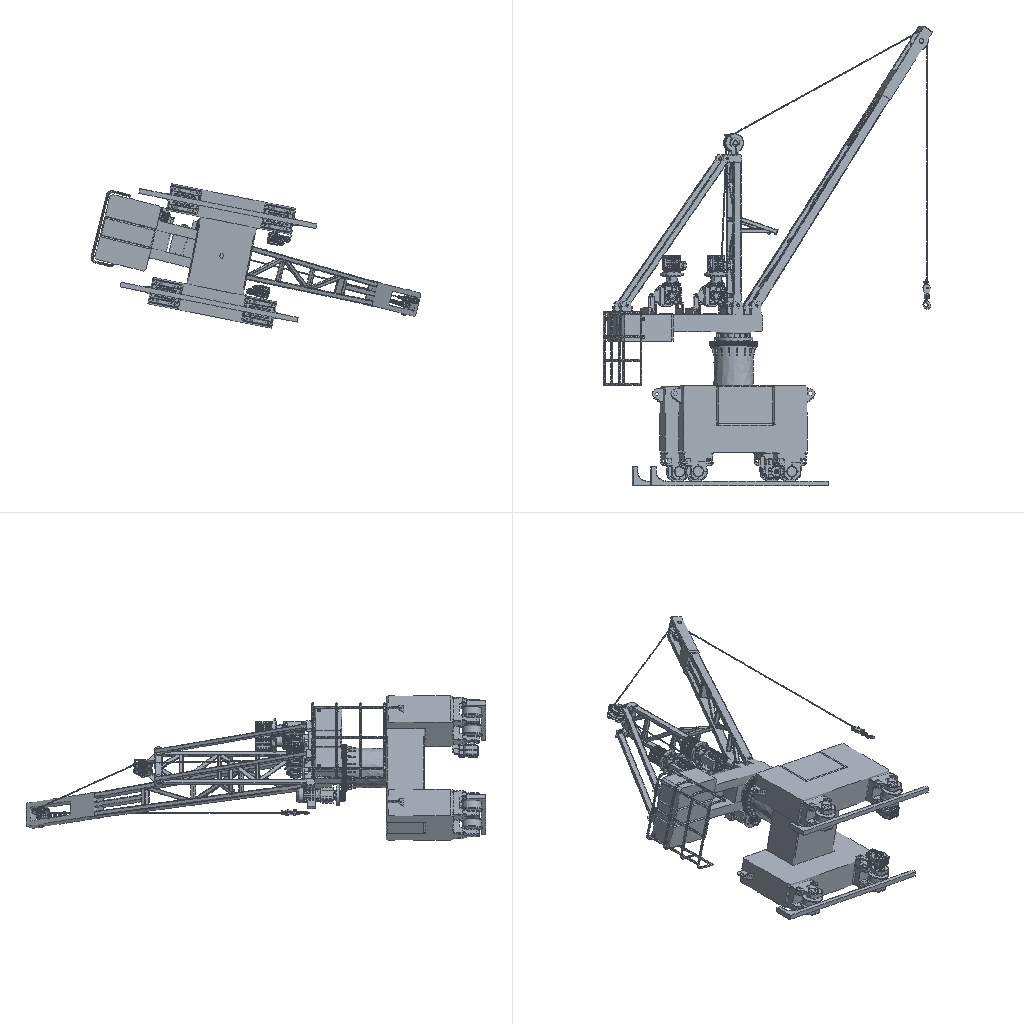Simulation study | ansys workbench
Set-up summary, first 208 of 6332 lines:
category,name,step,type,value,unit,region
solver,ansys_mapdl
solver,version,,,22.1
units,MPA,,stated
analysis,deck,,static,static
load_step,requested,,,1
analysis,nlgeom,,,False
mesh,nodes,,,2359965
mesh,elements,,,2475373
element_type,ANSYS 187 (type 1),,solid,1904
element_type,ANSYS 187 (type 2),,solid,1136
element_type,ANSYS 187 (type 3),,solid,1818
element_type,ANSYS 186 (type 4),,solid,45
element_type,ANSYS 186 (type 5),,solid,66
element_type,ANSYS 186 (type 6),,solid,36
element_type,ANSYS 186 (type 7),,solid,45
element_type,ANSYS 186 (type 8),,solid,66
element_type,ANSYS 186 (type 9),,solid,36
element_type,ANSYS 186 (type 10),,solid,36
element_type,ANSYS 186 (type 11),,solid,36
element_type,ANSYS 186 (type 12),,solid,45
element_type,ANSYS 186 (type 13),,solid,45
element_type,ANSYS 186 (type 14),,solid,66
element_type,ANSYS 186 (type 15),,solid,66
element_type,ANSYS 186 (type 16),,solid,42
element_type,ANSYS 186 (type 17),,solid,78
element_type,ANSYS 186 (type 18),,solid,36
element_type,ANSYS 186 (type 19),,solid,36
element_type,ANSYS 186 (type 20),,solid,42
element_type,ANSYS 186 (type 21),,solid,78
element_type,ANSYS 186 (type 22),,solid,42
element_type,ANSYS 186 (type 23),,solid,78
element_type,ANSYS 186 (type 24),,solid,78
element_type,ANSYS 186 (type 25),,solid,42
element_type,ANSYS 186 (type 26),,solid,36
element_type,ANSYS 186 (type 27),,solid,36
element_type,ANSYS 186 (type 28),,solid,45
element_type,ANSYS 186 (type 29),,solid,66
element_type,ANSYS 186 (type 30),,solid,35
element_type,ANSYS 186 (type 31),,solid,45
element_type,ANSYS 186 (type 32),,solid,66
element_type,ANSYS 186 (type 33),,solid,45
element_type,ANSYS 186 (type 34),,solid,66
element_type,ANSYS 186 (type 35),,solid,66
element_type,ANSYS 186 (type 36),,solid,45
element_type,ANSYS 186 (type 37),,solid,35
element_type,ANSYS 186 (type 38),,solid,32
element_type,ANSYS 186 (type 39),,solid,32
element_type,ANSYS 186 (type 40),,solid,24
element_type,ANSYS 186 (type 41),,solid,24
element_type,ANSYS 186 (type 42),,solid,24
element_type,ANSYS 186 (type 43),,solid,24
element_type,ANSYS 186 (type 44),,solid,32
element_type,ANSYS 186 (type 45),,solid,32
element_type,ANSYS 186 (type 46),,solid,42
element_type,ANSYS 186 (type 47),,solid,42
element_type,ANSYS 186 (type 48),,solid,42
element_type,ANSYS 186 (type 49),,solid,42
element_type,ANSYS 187 (type 50),,solid,3872
element_type,ANSYS 187 (type 51),,solid,4209
element_type,ANSYS 187 (type 52),,solid,188
element_type,ANSYS 187 (type 53),,solid,193
element_type,ANSYS 187 (type 54),,solid,189
element_type,ANSYS 187 (type 55),,solid,186
element_type,ANSYS 187 (type 56),,solid,187
element_type,ANSYS 187 (type 57),,solid,193
element_type,ANSYS 187 (type 58),,solid,186
element_type,ANSYS 187 (type 59),,solid,193
element_type,ANSYS 187 (type 60),,solid,2060
element_type,ANSYS 187 (type 61),,solid,1486
element_type,ANSYS 187 (type 62),,solid,1486
element_type,ANSYS 187 (type 63),,solid,2934
element_type,ANSYS 187 (type 64),,solid,158
element_type,ANSYS 187 (type 65),,solid,158
element_type,ANSYS 187 (type 66),,solid,158
element_type,ANSYS 187 (type 67),,solid,158
element_type,ANSYS 187 (type 68),,solid,6959
element_type,ANSYS 187 (type 69),,solid,9157
element_type,ANSYS 186 (type 70),,solid,1290
element_type,ANSYS 187 (type 71),,solid,9157
element_type,ANSYS 186 (type 72),,solid,38
element_type,ANSYS 186 (type 73),,solid,38
element_type,ANSYS 187 (type 74),,solid,493
element_type,ANSYS 187 (type 75),,solid,493
element_type,ANSYS 187 (type 76),,solid,811
element_type,ANSYS 187 (type 77),,solid,811
element_type,ANSYS 187 (type 78),,solid,811
element_type,ANSYS 187 (type 79),,solid,811
element_type,ANSYS 187 (type 80),,solid,811
element_type,ANSYS 187 (type 81),,solid,811
element_type,ANSYS 187 (type 82),,solid,811
element_type,ANSYS 187 (type 83),,solid,811
element_type,ANSYS 187 (type 84),,solid,576
element_type,ANSYS 187 (type 85),,solid,576
element_type,ANSYS 187 (type 86),,solid,576
element_type,ANSYS 186 (type 87),,solid,64
element_type,ANSYS 186 (type 88),,solid,64
element_type,ANSYS 186 (type 89),,solid,26
element_type,ANSYS 186 (type 90),,solid,26
element_type,ANSYS 186 (type 91),,solid,45
element_type,ANSYS 186 (type 92),,solid,45
element_type,ANSYS 186 (type 93),,solid,40
element_type,ANSYS 187 (type 94),,solid,5785
element_type,ANSYS 187 (type 95),,solid,6959
element_type,ANSYS 187 (type 96),,solid,6959
element_type,ANSYS 187 (type 97),,solid,9157
element_type,ANSYS 186 (type 98),,solid,1290
element_type,ANSYS 187 (type 99),,solid,9157
element_type,ANSYS 186 (type 100),,solid,38
element_type,ANSYS 186 (type 101),,solid,38
element_type,ANSYS 187 (type 102),,solid,493
element_type,ANSYS 187 (type 103),,solid,493
element_type,ANSYS 187 (type 104),,solid,811
element_type,ANSYS 187 (type 105),,solid,811
element_type,ANSYS 187 (type 106),,solid,811
element_type,ANSYS 187 (type 107),,solid,811
element_type,ANSYS 187 (type 108),,solid,811
element_type,ANSYS 187 (type 109),,solid,811
element_type,ANSYS 187 (type 110),,solid,811
element_type,ANSYS 187 (type 111),,solid,811
element_type,ANSYS 187 (type 112),,solid,576
element_type,ANSYS 187 (type 113),,solid,576
element_type,ANSYS 187 (type 114),,solid,576
element_type,ANSYS 186 (type 115),,solid,64
element_type,ANSYS 186 (type 116),,solid,64
element_type,ANSYS 186 (type 117),,solid,26
element_type,ANSYS 186 (type 118),,solid,26
element_type,ANSYS 186 (type 119),,solid,45
element_type,ANSYS 186 (type 120),,solid,45
element_type,ANSYS 186 (type 121),,solid,40
element_type,ANSYS 187 (type 122),,solid,5785
element_type,ANSYS 187 (type 123),,solid,6959
element_type,ANSYS 186 (type 124),,solid,156
element_type,ANSYS 186 (type 125),,solid,156
element_type,ANSYS 187 (type 126),,solid,6959
element_type,ANSYS 187 (type 127),,solid,9157
element_type,ANSYS 186 (type 128),,solid,1290
element_type,ANSYS 187 (type 129),,solid,9157
element_type,ANSYS 187 (type 130),,solid,9157
element_type,ANSYS 187 (type 131),,solid,2687
element_type,ANSYS 186 (type 132),,solid,38
element_type,ANSYS 186 (type 133),,solid,38
element_type,ANSYS 187 (type 134),,solid,493
element_type,ANSYS 187 (type 135),,solid,493
element_type,ANSYS 187 (type 136),,solid,576
element_type,ANSYS 187 (type 137),,solid,576
element_type,ANSYS 187 (type 138),,solid,576
element_type,ANSYS 186 (type 139),,solid,64
element_type,ANSYS 186 (type 140),,solid,64
element_type,ANSYS 186 (type 141),,solid,8
element_type,ANSYS 186 (type 142),,solid,26
element_type,ANSYS 186 (type 143),,solid,26
element_type,ANSYS 186 (type 144),,solid,45
element_type,ANSYS 186 (type 145),,solid,45
element_type,ANSYS 186 (type 146),,solid,40
element_type,ANSYS 187 (type 147),,solid,4056
element_type,ANSYS 187 (type 148),,solid,16584
element_type,ANSYS 187 (type 149),,solid,329
element_type,ANSYS 187 (type 150),,solid,1207
element_type,ANSYS 187 (type 151),,solid,5003
element_type,ANSYS 186 (type 152),,solid,25
element_type,ANSYS 186 (type 153),,solid,35
element_type,ANSYS 186 (type 154),,solid,160
element_type,ANSYS 186 (type 155),,solid,156
element_type,ANSYS 186 (type 156),,solid,156
element_type,ANSYS 187 (type 157),,solid,6959
element_type,ANSYS 187 (type 158),,solid,9157
element_type,ANSYS 186 (type 159),,solid,1290
element_type,ANSYS 187 (type 160),,solid,9157
element_type,ANSYS 187 (type 161),,solid,9157
element_type,ANSYS 187 (type 162),,solid,2687
element_type,ANSYS 186 (type 163),,solid,38
element_type,ANSYS 186 (type 164),,solid,38
element_type,ANSYS 187 (type 165),,solid,493
element_type,ANSYS 187 (type 166),,solid,493
element_type,ANSYS 187 (type 167),,solid,576
element_type,ANSYS 187 (type 168),,solid,576
element_type,ANSYS 187 (type 169),,solid,576
element_type,ANSYS 186 (type 170),,solid,64
element_type,ANSYS 186 (type 171),,solid,64
element_type,ANSYS 186 (type 172),,solid,8
element_type,ANSYS 186 (type 173),,solid,26
element_type,ANSYS 186 (type 174),,solid,26
element_type,ANSYS 186 (type 175),,solid,45
element_type,ANSYS 186 (type 176),,solid,45
element_type,ANSYS 186 (type 177),,solid,40
element_type,ANSYS 187 (type 178),,solid,4056
element_type,ANSYS 187 (type 179),,solid,16584
element_type,ANSYS 187 (type 180),,solid,329
element_type,ANSYS 187 (type 181),,solid,1207
element_type,ANSYS 187 (type 182),,solid,5003
element_type,ANSYS 186 (type 183),,solid,25
element_type,ANSYS 186 (type 184),,solid,35
element_type,ANSYS 186 (type 185),,solid,160
element_type,ANSYS 187 (type 186),,solid,1135
element_type,ANSYS 186 (type 187),,solid,906
element_type,ANSYS 187 (type 188),,solid,12141
element_type,ANSYS 187 (type 189),,solid,12141
element_type,ANSYS 186 (type 190),,solid,906
element_type,ANSYS 186 (type 191),,solid,906
element_type,ANSYS 187 (type 192),,solid,696
element_type,ANSYS 187 (type 193),,solid,696
element_type,ANSYS 187 (type 194),,solid,696
element_type,ANSYS 187 (type 195),,solid,696
element_type,ANSYS 186 (type 196),,solid,132
element_type,ANSYS 187 (type 197),,solid,1726
element_type,ANSYS 187 (type 198),,solid,1726
element_type,ANSYS 187 (type 199),,solid,1639
Results summary:
result,analysis,,,static
result,last_loadstep,,,1
result,primary field,,,displacement
result,reaction total,1,FX,4.9e-05,N
result,reaction total,1,FY,500000,N
result,reaction total,1,FZ,-0.000588,N
result,mass,,,7.647,"NMM: mm, ton, N, s, mV, mA, degC"